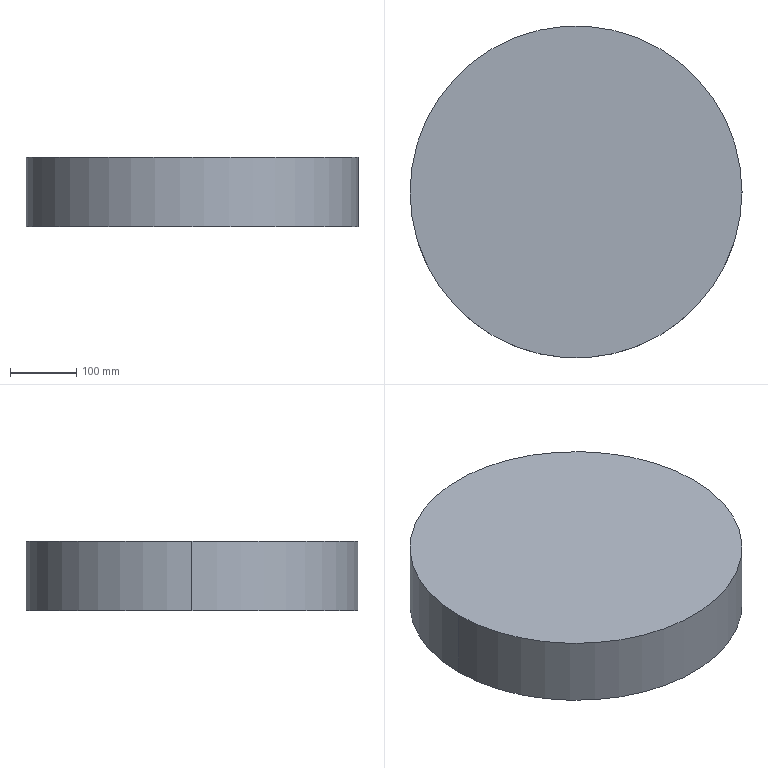Part | SolidWorks | features Extrusion 1 | 1 solid | 4 faces | box 500 x 500 x 105 mm | volume 20616702 mm3 | cylinder 2 | plane 2 | commonest cylinder face diameters 500 x2
STEP:
#1=CARTESIAN_POINT('',(250.,0.,105.));
#2=VERTEX_POINT('',#1);
#3=CARTESIAN_POINT('',(-250.,0.,105.));
#4=VERTEX_POINT('',#3);
#5=CARTESIAN_POINT('',(0.,0.,105.));
#6=DIRECTION('',(0.,0.,1.));
#7=DIRECTION('',(1.,0.,0.));
#8=AXIS2_PLACEMENT_3D('',#5,#6,#7);
#9=CIRCLE('',#8,250.);
#10=EDGE_CURVE('',#2,#4,#9,.T.);
#11=ORIENTED_EDGE('',*,*,#10,.F.);
#12=CARTESIAN_POINT('',(250.,0.,0.));
#13=VERTEX_POINT('',#12);
#14=CARTESIAN_POINT('',(250.,0.,105.));
#15=DIRECTION('',(0.,0.,-1.));
#16=VECTOR('',#15,1000.);
#17=LINE('',#14,#16);
#18=EDGE_CURVE('',#2,#13,#17,.T.);
#19=ORIENTED_EDGE('',*,*,#18,.T.);
#20=CARTESIAN_POINT('',(-250.,0.,0.));
#21=VERTEX_POINT('',#20);
#22=CARTESIAN_POINT('',(0.,0.,0.));
#23=DIRECTION('',(0.,0.,1.));
#24=DIRECTION('',(1.,0.,0.));
#25=AXIS2_PLACEMENT_3D('',#22,#23,#24);
#26=CIRCLE('',#25,250.);
#27=EDGE_CURVE('',#13,#21,#26,.T.);
#28=ORIENTED_EDGE('',*,*,#27,.T.);
#29=CARTESIAN_POINT('',(-250.,0.,105.));
#30=DIRECTION('',(0.,0.,-1.));
#31=VECTOR('',#30,1000.);
#32=LINE('',#29,#31);
#33=EDGE_CURVE('',#4,#21,#32,.T.);
#34=ORIENTED_EDGE('',*,*,#33,.F.);
#35=EDGE_LOOP('',(#11,#19,#28,#34));
#36=FACE_OUTER_BOUND('',#35,.T.);
#37=CARTESIAN_POINT('',(0.,0.,105.));
#38=DIRECTION('',(0.,0.,-1.));
#39=DIRECTION('',(-1.,0.,0.));
#40=AXIS2_PLACEMENT_3D('',#37,#38,#39);
#41=CYLINDRICAL_SURFACE('',#40,250.);
#42=ADVANCED_FACE('',(#36),#41,.T.);
#43=ORIENTED_EDGE('',*,*,#18,.F.);
#44=CARTESIAN_POINT('',(0.,0.,105.));
#45=DIRECTION('',(0.,0.,1.));
#46=DIRECTION('',(1.,0.,0.));
#47=AXIS2_PLACEMENT_3D('',#44,#45,#46);
#48=CIRCLE('',#47,250.);
#49=EDGE_CURVE('',#4,#2,#48,.T.);
#50=ORIENTED_EDGE('',*,*,#49,.F.);
#51=ORIENTED_EDGE('',*,*,#33,.T.);
#52=CARTESIAN_POINT('',(0.,0.,0.));
#53=DIRECTION('',(0.,0.,1.));
#54=DIRECTION('',(1.,0.,0.));
#55=AXIS2_PLACEMENT_3D('',#52,#53,#54);
#56=CIRCLE('',#55,250.);
#57=EDGE_CURVE('',#21,#13,#56,.T.);
#58=ORIENTED_EDGE('',*,*,#57,.T.);
#59=EDGE_LOOP('',(#43,#50,#51,#58));
#60=FACE_OUTER_BOUND('',#59,.T.);
#61=CARTESIAN_POINT('',(0.,0.,105.));
#62=DIRECTION('',(0.,0.,-1.));
#63=DIRECTION('',(-1.,0.,0.));
#64=AXIS2_PLACEMENT_3D('',#61,#62,#63);
#65=CYLINDRICAL_SURFACE('',#64,250.);
#66=ADVANCED_FACE('',(#60),#65,.T.);
#67=ORIENTED_EDGE('',*,*,#49,.T.);
#68=ORIENTED_EDGE('',*,*,#10,.T.);
#69=EDGE_LOOP('',(#67,#68));
#70=FACE_OUTER_BOUND('',#69,.T.);
#71=CARTESIAN_POINT('',(0.,0.,105.));
#72=DIRECTION('',(0.,0.,1.));
#73=DIRECTION('',(1.,0.,0.));
#74=AXIS2_PLACEMENT_3D('',#71,#72,#73);
#75=PLANE('',#74);
#76=ADVANCED_FACE('',(#70),#75,.T.);
#77=ORIENTED_EDGE('',*,*,#57,.F.);
#78=ORIENTED_EDGE('',*,*,#27,.F.);
#79=EDGE_LOOP('',(#77,#78));
#80=FACE_OUTER_BOUND('',#79,.T.);
#81=CARTESIAN_POINT('',(0.,0.,0.));
#82=DIRECTION('',(0.,0.,1.));
#83=DIRECTION('',(1.,0.,0.));
#84=AXIS2_PLACEMENT_3D('',#81,#82,#83);
#85=PLANE('',#84);
#86=ADVANCED_FACE('',(#80),#85,.F.);
#87=CLOSED_SHELL('',(#42,#66,#76,#86));
#88=MANIFOLD_SOLID_BREP('',#87);
#89=CARTESIAN_POINT('',(0.,0.,0.));
#90=DIRECTION('',(0.,0.,1.));
#91=DIRECTION('',(1.,0.,0.));
#92=AXIS2_PLACEMENT_3D('',#89,#90,#91);
#93=(LENGTH_UNIT()NAMED_UNIT(*)SI_UNIT(.MILLI.,.METRE.));
#94=UNCERTAINTY_MEASURE_WITH_UNIT(LENGTH_MEASURE(0.00001),#93,'','');
#95=(NAMED_UNIT(*)PLANE_ANGLE_UNIT()SI_UNIT($,.RADIAN.));
#96=(NAMED_UNIT(*)SI_UNIT($,.STERADIAN.)SOLID_ANGLE_UNIT());
#97=(GEOMETRIC_REPRESENTATION_CONTEXT(3)GLOBAL_UNCERTAINTY_ASSIGNED_CONTEXT((#94))GLOBAL_UNIT_ASSIGNED_CONTEXT((#93,#95,#96))REPRESENTATION_CONTEXT('',''));
#98=ADVANCED_BREP_SHAPE_REPRESENTATION('',(#88,#92),#97);